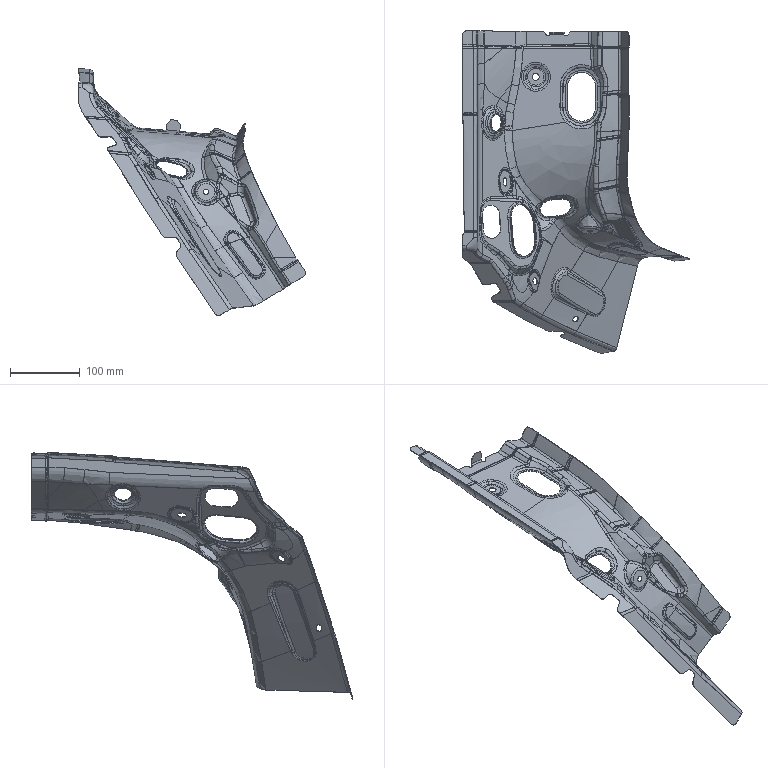Part | STEP file | FNA5401753 | 1 solid | 1240 faces | box 326.803 x 462.989 x 355.554 mm | volume 121540 mm3 | spline 1068 | cylinder 76 | plane 60 | other 28 | sphere 4 | torus 4 | commonest cylinder face diameters 12 x10 10.4 x9 7 x4 10 x4 280 x4 281.6 x4